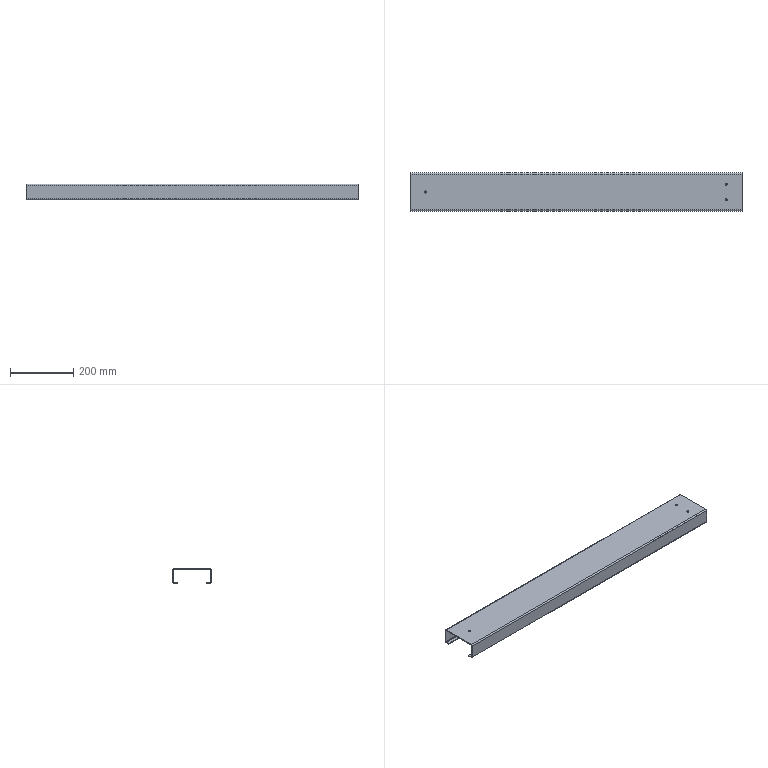Part | SolidWorks | features BaseBody 1 | 1 solid | 44 faces | box 1046 x 120 x 50 mm | volume 733077 mm3 | plane 30 | cylinder 14 | commonest cylinder face diameters 6.5 x6 2 x4 8 x4
STEP:
#1=CARTESIAN_POINT('',(469.75,25.,-3.));
#2=VERTEX_POINT('',#1);
#3=CARTESIAN_POINT('',(469.75,25.,0.));
#4=VERTEX_POINT('',#3);
#5=CARTESIAN_POINT('',(469.75,25.,-3.));
#6=DIRECTION('',(0.,0.,1.));
#7=VECTOR('',#6,1000.);
#8=LINE('',#5,#7);
#9=EDGE_CURVE('',#2,#4,#8,.T.);
#10=ORIENTED_EDGE('',*,*,#9,.F.);
#11=CARTESIAN_POINT('',(476.25,25.,-3.));
#12=VERTEX_POINT('',#11);
#13=CARTESIAN_POINT('',(473.,25.,-3.));
#14=DIRECTION('',(0.,0.,1.));
#15=DIRECTION('',(1.,0.,0.));
#16=AXIS2_PLACEMENT_3D('',#13,#14,#15);
#17=CIRCLE('',#16,3.25);
#18=EDGE_CURVE('',#12,#2,#17,.T.);
#19=ORIENTED_EDGE('',*,*,#18,.F.);
#20=CARTESIAN_POINT('',(476.25,25.,0.));
#21=VERTEX_POINT('',#20);
#22=CARTESIAN_POINT('',(476.25,25.,-3.));
#23=DIRECTION('',(0.,0.,1.));
#24=VECTOR('',#23,1000.);
#25=LINE('',#22,#24);
#26=EDGE_CURVE('',#12,#21,#25,.T.);
#27=ORIENTED_EDGE('',*,*,#26,.T.);
#28=CARTESIAN_POINT('',(473.,25.,0.));
#29=DIRECTION('',(0.,0.,1.));
#30=DIRECTION('',(1.,0.,0.));
#31=AXIS2_PLACEMENT_3D('',#28,#29,#30);
#32=CIRCLE('',#31,3.25);
#33=EDGE_CURVE('',#21,#4,#32,.T.);
#34=ORIENTED_EDGE('',*,*,#33,.T.);
#35=EDGE_LOOP('',(#10,#19,#27,#34));
#36=FACE_OUTER_BOUND('',#35,.T.);
#37=CARTESIAN_POINT('',(473.,25.,-3.));
#38=DIRECTION('',(0.,0.,1.));
#39=DIRECTION('',(1.,0.,0.));
#40=AXIS2_PLACEMENT_3D('',#37,#38,#39);
#41=CYLINDRICAL_SURFACE('',#40,3.25);
#42=ADVANCED_FACE('',(#36),#41,.F.);
#43=CARTESIAN_POINT('',(469.75,-25.,-3.));
#44=VERTEX_POINT('',#43);
#45=CARTESIAN_POINT('',(469.75,-25.,0.));
#46=VERTEX_POINT('',#45);
#47=CARTESIAN_POINT('',(469.75,-25.,-3.));
#48=DIRECTION('',(0.,0.,1.));
#49=VECTOR('',#48,1000.);
#50=LINE('',#47,#49);
#51=EDGE_CURVE('',#44,#46,#50,.T.);
#52=ORIENTED_EDGE('',*,*,#51,.F.);
#53=CARTESIAN_POINT('',(476.25,-25.,-3.));
#54=VERTEX_POINT('',#53);
#55=CARTESIAN_POINT('',(473.,-25.,-3.));
#56=DIRECTION('',(0.,0.,1.));
#57=DIRECTION('',(1.,0.,0.));
#58=AXIS2_PLACEMENT_3D('',#55,#56,#57);
#59=CIRCLE('',#58,3.25);
#60=EDGE_CURVE('',#54,#44,#59,.T.);
#61=ORIENTED_EDGE('',*,*,#60,.F.);
#62=CARTESIAN_POINT('',(476.25,-25.,0.));
#63=VERTEX_POINT('',#62);
#64=CARTESIAN_POINT('',(476.25,-25.,-3.));
#65=DIRECTION('',(0.,0.,1.));
#66=VECTOR('',#65,1000.);
#67=LINE('',#64,#66);
#68=EDGE_CURVE('',#54,#63,#67,.T.);
#69=ORIENTED_EDGE('',*,*,#68,.T.);
#70=CARTESIAN_POINT('',(473.,-25.,0.));
#71=DIRECTION('',(0.,0.,1.));
#72=DIRECTION('',(1.,0.,0.));
#73=AXIS2_PLACEMENT_3D('',#70,#71,#72);
#74=CIRCLE('',#73,3.25);
#75=EDGE_CURVE('',#63,#46,#74,.T.);
#76=ORIENTED_EDGE('',*,*,#75,.T.);
#77=EDGE_LOOP('',(#52,#61,#69,#76));
#78=FACE_OUTER_BOUND('',#77,.T.);
#79=CARTESIAN_POINT('',(473.,-25.,-3.));
#80=DIRECTION('',(0.,0.,1.));
#81=DIRECTION('',(1.,0.,0.));
#82=AXIS2_PLACEMENT_3D('',#79,#80,#81);
#83=CYLINDRICAL_SURFACE('',#82,3.25);
#84=ADVANCED_FACE('',(#78),#83,.F.);
#85=CARTESIAN_POINT('',(-476.25,0.,-3.));
#86=VERTEX_POINT('',#85);
#87=CARTESIAN_POINT('',(-476.25,0.,0.));
#88=VERTEX_POINT('',#87);
#89=CARTESIAN_POINT('',(-476.25,0.,-3.));
#90=DIRECTION('',(0.,0.,1.));
#91=VECTOR('',#90,1000.);
#92=LINE('',#89,#91);
#93=EDGE_CURVE('',#86,#88,#92,.T.);
#94=ORIENTED_EDGE('',*,*,#93,.F.);
#95=CARTESIAN_POINT('',(-469.75,0.,-3.));
#96=VERTEX_POINT('',#95);
#97=CARTESIAN_POINT('',(-473.,0.,-3.));
#98=DIRECTION('',(0.,0.,1.));
#99=DIRECTION('',(1.,0.,0.));
#100=AXIS2_PLACEMENT_3D('',#97,#98,#99);
#101=CIRCLE('',#100,3.25);
#102=EDGE_CURVE('',#96,#86,#101,.T.);
#103=ORIENTED_EDGE('',*,*,#102,.F.);
#104=CARTESIAN_POINT('',(-469.75,0.,0.));
#105=VERTEX_POINT('',#104);
#106=CARTESIAN_POINT('',(-469.75,0.,-3.));
#107=DIRECTION('',(0.,0.,1.));
#108=VECTOR('',#107,1000.);
#109=LINE('',#106,#108);
#110=EDGE_CURVE('',#96,#105,#109,.T.);
#111=ORIENTED_EDGE('',*,*,#110,.T.);
#112=CARTESIAN_POINT('',(-473.,0.,0.));
#113=DIRECTION('',(0.,0.,1.));
#114=DIRECTION('',(1.,0.,0.));
#115=AXIS2_PLACEMENT_3D('',#112,#113,#114);
#116=CIRCLE('',#115,3.25);
#117=EDGE_CURVE('',#105,#88,#116,.T.);
#118=ORIENTED_EDGE('',*,*,#117,.T.);
#119=EDGE_LOOP('',(#94,#103,#111,#118));
#120=FACE_OUTER_BOUND('',#119,.T.);
#121=CARTESIAN_POINT('',(-473.,0.,-3.));
#122=DIRECTION('',(0.,0.,1.));
#123=DIRECTION('',(1.,0.,0.));
#124=AXIS2_PLACEMENT_3D('',#121,#122,#123);
#125=CYLINDRICAL_SURFACE('',#124,3.25);
#126=ADVANCED_FACE('',(#120),#125,.F.);
#127=CARTESIAN_POINT('',(523.,45.,-47.));
#128=VERTEX_POINT('',#127);
#129=CARTESIAN_POINT('',(-523.,45.,-47.));
#130=VERTEX_POINT('',#129);
#131=CARTESIAN_POINT('',(-523.,45.,-47.));
#132=DIRECTION('',(-1.,0.,0.));
#133=VECTOR('',#132,1000.);
#134=LINE('',#131,#133);
#135=EDGE_CURVE('',#128,#130,#134,.T.);
#136=ORIENTED_EDGE('',*,*,#135,.T.);
#137=CARTESIAN_POINT('',(-523.,45.,-50.));
#138=VERTEX_POINT('',#137);
#139=CARTESIAN_POINT('',(-523.,45.,-50.));
#140=DIRECTION('',(0.,0.,1.));
#141=VECTOR('',#140,1000.);
#142=LINE('',#139,#141);
#143=EDGE_CURVE('',#138,#130,#142,.T.);
#144=ORIENTED_EDGE('',*,*,#143,.F.);
#145=CARTESIAN_POINT('',(523.,45.,-50.));
#146=VERTEX_POINT('',#145);
#147=CARTESIAN_POINT('',(0.,45.,-50.));
#148=DIRECTION('',(-1.,0.,0.));
#149=VECTOR('',#148,1000.);
#150=LINE('',#147,#149);
#151=EDGE_CURVE('',#146,#138,#150,.T.);
#152=ORIENTED_EDGE('',*,*,#151,.F.);
#153=CARTESIAN_POINT('',(523.,45.,-50.));
#154=DIRECTION('',(0.,0.,1.));
#155=VECTOR('',#154,1000.);
#156=LINE('',#153,#155);
#157=EDGE_CURVE('',#146,#128,#156,.T.);
#158=ORIENTED_EDGE('',*,*,#157,.T.);
#159=EDGE_LOOP('',(#136,#144,#152,#158));
#160=FACE_OUTER_BOUND('',#159,.T.);
#161=CARTESIAN_POINT('',(-523.,45.,-50.));
#162=DIRECTION('',(0.,1.,0.));
#163=DIRECTION('',(0.,0.,-1.));
#164=AXIS2_PLACEMENT_3D('',#161,#162,#163);
#165=PLANE('',#164);
#166=ADVANCED_FACE('',(#160),#165,.F.);
#167=CARTESIAN_POINT('',(523.,56.,-47.));
#168=VERTEX_POINT('',#167);
#169=CARTESIAN_POINT('',(523.,45.,-47.));
#170=DIRECTION('',(0.,-1.,0.));
#171=VECTOR('',#170,1000.);
#172=LINE('',#169,#171);
#173=EDGE_CURVE('',#168,#128,#172,.T.);
#174=ORIENTED_EDGE('',*,*,#173,.F.);
#175=CARTESIAN_POINT('',(-523.,56.,-47.));
#176=VERTEX_POINT('',#175);
#177=CARTESIAN_POINT('',(-523.,56.,-47.));
#178=DIRECTION('',(1.,0.,0.));
#179=VECTOR('',#178,1000.);
#180=LINE('',#177,#179);
#181=EDGE_CURVE('',#176,#168,#180,.T.);
#182=ORIENTED_EDGE('',*,*,#181,.F.);
#183=CARTESIAN_POINT('',(-523.,57.,-47.));
#184=DIRECTION('',(0.,1.,0.));
#185=VECTOR('',#184,1000.);
#186=LINE('',#183,#185);
#187=EDGE_CURVE('',#130,#176,#186,.T.);
#188=ORIENTED_EDGE('',*,*,#187,.F.);
#189=ORIENTED_EDGE('',*,*,#135,.F.);
#190=EDGE_LOOP('',(#174,#182,#188,#189));
#191=FACE_OUTER_BOUND('',#190,.T.);
#192=CARTESIAN_POINT('',(0.,0.,-47.));
#193=DIRECTION('',(0.,0.,1.));
#194=DIRECTION('',(0.,-1.,0.));
#195=AXIS2_PLACEMENT_3D('',#192,#193,#194);
#196=PLANE('',#195);
#197=ADVANCED_FACE('',(#191),#196,.T.);
#198=CARTESIAN_POINT('',(523.,56.,-50.));
#199=VERTEX_POINT('',#198);
#200=CARTESIAN_POINT('',(-523.,56.,-50.));
#201=VERTEX_POINT('',#200);
#202=CARTESIAN_POINT('',(-523.,56.,-50.));
#203=DIRECTION('',(-1.,0.,0.));
#204=VECTOR('',#203,1000.);
#205=LINE('',#202,#204);
#206=EDGE_CURVE('',#199,#201,#205,.T.);
#207=ORIENTED_EDGE('',*,*,#206,.F.);
#208=CARTESIAN_POINT('',(523.,0.,-50.));
#209=DIRECTION('',(0.,-1.,0.));
#210=VECTOR('',#209,1000.);
#211=LINE('',#208,#210);
#212=EDGE_CURVE('',#199,#146,#211,.T.);
#213=ORIENTED_EDGE('',*,*,#212,.T.);
#214=ORIENTED_EDGE('',*,*,#151,.T.);
#215=CARTESIAN_POINT('',(-523.,0.,-50.));
#216=DIRECTION('',(0.,1.,0.));
#217=VECTOR('',#216,1000.);
#218=LINE('',#215,#217);
#219=EDGE_CURVE('',#138,#201,#218,.T.);
#220=ORIENTED_EDGE('',*,*,#219,.T.);
#221=EDGE_LOOP('',(#207,#213,#214,#220));
#222=FACE_OUTER_BOUND('',#221,.T.);
#223=CARTESIAN_POINT('',(0.,0.,-50.));
#224=DIRECTION('',(0.,0.,1.));
#225=DIRECTION('',(0.,-1.,0.));
#226=AXIS2_PLACEMENT_3D('',#223,#224,#225);
#227=PLANE('',#226);
#228=ADVANCED_FACE('',(#222),#227,.F.);
#229=CARTESIAN_POINT('',(-523.,56.,-50.));
#230=DIRECTION('',(0.,0.,-1.));
#231=VECTOR('',#230,1000.);
#232=LINE('',#229,#231);
#233=EDGE_CURVE('',#176,#201,#232,.T.);
#234=ORIENTED_EDGE('',*,*,#233,.T.);
#235=ORIENTED_EDGE('',*,*,#219,.F.);
#236=ORIENTED_EDGE('',*,*,#143,.T.);
#237=ORIENTED_EDGE('',*,*,#187,.T.);
#238=EDGE_LOOP('',(#234,#235,#236,#237));
#239=FACE_OUTER_BOUND('',#238,.T.);
#240=CARTESIAN_POINT('',(-523.,57.,-50.));
#241=DIRECTION('',(1.,0.,0.));
#242=DIRECTION('',(0.,1.,0.));
#243=AXIS2_PLACEMENT_3D('',#240,#241,#242);
#244=PLANE('',#243);
#245=ADVANCED_FACE('',(#239),#244,.F.);
#246=CARTESIAN_POINT('',(523.,56.,-47.));
#247=DIRECTION('',(0.,0.,-1.));
#248=VECTOR('',#247,1000.);
#249=LINE('',#246,#248);
#250=EDGE_CURVE('',#168,#199,#249,.T.);
#251=ORIENTED_EDGE('',*,*,#250,.F.);
#252=ORIENTED_EDGE('',*,*,#173,.T.);
#253=ORIENTED_EDGE('',*,*,#157,.F.);
#254=ORIENTED_EDGE('',*,*,#212,.F.);
#255=EDGE_LOOP('',(#251,#252,#253,#254));
#256=FACE_OUTER_BOUND('',#255,.T.);
#257=CARTESIAN_POINT('',(523.,45.,-50.));
#258=DIRECTION('',(-1.,0.,0.));
#259=DIRECTION('',(0.,0.,1.));
#260=AXIS2_PLACEMENT_3D('',#257,#258,#259);
#261=PLANE('',#260);
#262=ADVANCED_FACE('',(#256),#261,.F.);
#263=CARTESIAN_POINT('',(523.,57.,-46.));
#264=VERTEX_POINT('',#263);
#265=CARTESIAN_POINT('',(-523.,57.,-46.));
#266=VERTEX_POINT('',#265);
#267=CARTESIAN_POINT('',(523.,57.,-46.));
#268=DIRECTION('',(-1.,0.,0.));
#269=VECTOR('',#268,1000.);
#270=LINE('',#267,#269);
#271=EDGE_CURVE('',#264,#266,#270,.T.);
#272=ORIENTED_EDGE('',*,*,#271,.T.);
#273=CARTESIAN_POINT('',(-523.,56.,-46.));
#274=DIRECTION('',(-1.,0.,0.));
#275=DIRECTION('',(0.,0.,-1.));
#276=AXIS2_PLACEMENT_3D('',#273,#274,#275);
#277=CIRCLE('',#276,1.);
#278=EDGE_CURVE('',#266,#176,#277,.T.);
#279=ORIENTED_EDGE('',*,*,#278,.T.);
#280=ORIENTED_EDGE('',*,*,#181,.T.);
#281=CARTESIAN_POINT('',(523.,56.,-46.));
#282=DIRECTION('',(1.,0.,0.));
#283=DIRECTION('',(0.,0.,-1.));
#284=AXIS2_PLACEMENT_3D('',#281,#282,#283);
#285=CIRCLE('',#284,1.);
#286=EDGE_CURVE('',#168,#264,#285,.T.);
#287=ORIENTED_EDGE('',*,*,#286,.T.);
#288=EDGE_LOOP('',(#272,#279,#280,#287));
#289=FACE_OUTER_BOUND('',#288,.T.);
#290=CARTESIAN_POINT('',(523.,56.,-46.));
#291=DIRECTION('',(1.,0.,0.));
#292=DIRECTION('',(0.,0.,-1.));
#293=AXIS2_PLACEMENT_3D('',#290,#291,#292);
#294=CYLINDRICAL_SURFACE('',#293,1.);
#295=ADVANCED_FACE('',(#289),#294,.F.);
#296=CARTESIAN_POINT('',(523.,60.,-46.));
#297=VERTEX_POINT('',#296);
#298=CARTESIAN_POINT('',(-523.,60.,-46.));
#299=VERTEX_POINT('',#298);
#300=CARTESIAN_POINT('',(523.,60.,-46.));
#301=DIRECTION('',(-1.,0.,0.));
#302=VECTOR('',#301,1000.);
#303=LINE('',#300,#302);
#304=EDGE_CURVE('',#297,#299,#303,.T.);
#305=ORIENTED_EDGE('',*,*,#304,.F.);
#306=CARTESIAN_POINT('',(523.,56.,-46.));
#307=DIRECTION('',(1.,0.,0.));
#308=DIRECTION('',(0.,0.,-1.));
#309=AXIS2_PLACEMENT_3D('',#306,#307,#308);
#310=CIRCLE('',#309,4.);
#311=EDGE_CURVE('',#199,#297,#310,.T.);
#312=ORIENTED_EDGE('',*,*,#311,.F.);
#313=ORIENTED_EDGE('',*,*,#206,.T.);
#314=CARTESIAN_POINT('',(-523.,56.,-46.));
#315=DIRECTION('',(-1.,0.,0.));
#316=DIRECTION('',(0.,0.,-1.));
#317=AXIS2_PLACEMENT_3D('',#314,#315,#316);
#318=CIRCLE('',#317,4.);
#319=EDGE_CURVE('',#299,#201,#318,.T.);
#320=ORIENTED_EDGE('',*,*,#319,.F.);
#321=EDGE_LOOP('',(#305,#312,#313,#320));
#322=FACE_OUTER_BOUND('',#321,.T.);
#323=CARTESIAN_POINT('',(523.,56.,-46.));
#324=DIRECTION('',(1.,0.,0.));
#325=DIRECTION('',(0.,0.,-1.));
#326=AXIS2_PLACEMENT_3D('',#323,#324,#325);
#327=CYLINDRICAL_SURFACE('',#326,4.);
#328=ADVANCED_FACE('',(#322),#327,.T.);
#329=ORIENTED_EDGE('',*,*,#286,.F.);
#330=ORIENTED_EDGE('',*,*,#250,.T.);
#331=ORIENTED_EDGE('',*,*,#311,.T.);
#332=CARTESIAN_POINT('',(523.,57.,-46.));
#333=DIRECTION('',(0.,1.,0.));
#334=VECTOR('',#333,1000.);
#335=LINE('',#332,#334);
#336=EDGE_CURVE('',#264,#297,#335,.T.);
#337=ORIENTED_EDGE('',*,*,#336,.F.);
#338=EDGE_LOOP('',(#329,#330,#331,#337));
#339=FACE_OUTER_BOUND('',#338,.T.);
#340=CARTESIAN_POINT('',(523.,56.,-46.));
#341=DIRECTION('',(-1.,0.,0.));
#342=DIRECTION('',(0.,0.,1.));
#343=AXIS2_PLACEMENT_3D('',#340,#341,#342);
#344=PLANE('',#343);
#345=ADVANCED_FACE('',(#339),#344,.F.);
#346=ORIENTED_EDGE('',*,*,#233,.F.);
#347=ORIENTED_EDGE('',*,*,#278,.F.);
#348=CARTESIAN_POINT('',(-523.,57.,-46.));
#349=DIRECTION('',(0.,1.,0.));
#350=VECTOR('',#349,1000.);
#351=LINE('',#348,#350);
#352=EDGE_CURVE('',#266,#299,#351,.T.);
#353=ORIENTED_EDGE('',*,*,#352,.T.);
#354=ORIENTED_EDGE('',*,*,#319,.T.);
#355=EDGE_LOOP('',(#346,#347,#353,#354));
#356=FACE_OUTER_BOUND('',#355,.T.);
#357=CARTESIAN_POINT('',(-523.,56.,-46.));
#358=DIRECTION('',(-1.,0.,0.));
#359=DIRECTION('',(0.,0.,1.));
#360=AXIS2_PLACEMENT_3D('',#357,#358,#359);
#361=PLANE('',#360);
#362=ADVANCED_FACE('',(#356),#361,.T.);
#363=CARTESIAN_POINT('',(-523.,-45.,-47.));
#364=VERTEX_POINT('',#363);
#365=CARTESIAN_POINT('',(523.,-45.,-47.));
#366=VERTEX_POINT('',#365);
#367=CARTESIAN_POINT('',(523.,-45.,-47.));
#368=DIRECTION('',(1.,0.,0.));
#369=VECTOR('',#368,1000.);
#370=LINE('',#367,#369);
#371=EDGE_CURVE('',#364,#366,#370,.T.);
#372=ORIENTED_EDGE('',*,*,#371,.T.);
#373=CARTESIAN_POINT('',(523.,-45.,-50.));
#374=VERTEX_POINT('',#373);
#375=CARTESIAN_POINT('',(523.,-45.,-50.));
#376=DIRECTION('',(0.,0.,1.));
#377=VECTOR('',#376,1000.);
#378=LINE('',#375,#377);
#379=EDGE_CURVE('',#374,#366,#378,.T.);
#380=ORIENTED_EDGE('',*,*,#379,.F.);
#381=CARTESIAN_POINT('',(-523.,-45.,-50.));
#382=VERTEX_POINT('',#381);
#383=CARTESIAN_POINT('',(0.,-45.,-50.));
#384=DIRECTION('',(1.,0.,0.));
#385=VECTOR('',#384,1000.);
#386=LINE('',#383,#385);
#387=EDGE_CURVE('',#382,#374,#386,.T.);
#388=ORIENTED_EDGE('',*,*,#387,.F.);
#389=CARTESIAN_POINT('',(-523.,-45.,-50.));
#390=DIRECTION('',(0.,0.,1.));
#391=VECTOR('',#390,1000.);
#392=LINE('',#389,#391);
#393=EDGE_CURVE('',#382,#364,#392,.T.);
#394=ORIENTED_EDGE('',*,*,#393,.T.);
#395=EDGE_LOOP('',(#372,#380,#388,#394));
#396=FACE_OUTER_BOUND('',#395,.T.);
#397=CARTESIAN_POINT('',(523.,-45.,-50.));
#398=DIRECTION('',(0.,-1.,0.));
#399=DIRECTION('',(-1.,0.,0.));
#400=AXIS2_PLACEMENT_3D('',#397,#398,#399);
#401=PLANE('',#400);
#402=ADVANCED_FACE('',(#396),#401,.F.);
#403=CARTESIAN_POINT('',(-523.,-56.,-47.));
#404=VERTEX_POINT('',#403);
#405=CARTESIAN_POINT('',(-523.,-45.,-47.));
#406=DIRECTION('',(0.,1.,0.));
#407=VECTOR('',#406,1000.);
#408=LINE('',#405,#407);
#409=EDGE_CURVE('',#404,#364,#408,.T.);
#410=ORIENTED_EDGE('',*,*,#409,.F.);
#411=CARTESIAN_POINT('',(523.,-56.,-47.));
#412=VERTEX_POINT('',#411);
#413=CARTESIAN_POINT('',(523.,-56.,-47.));
#414=DIRECTION('',(-1.,0.,0.));
#415=VECTOR('',#414,1000.);
#416=LINE('',#413,#415);
#417=EDGE_CURVE('',#412,#404,#416,.T.);
#418=ORIENTED_EDGE('',*,*,#417,.F.);
#419=CARTESIAN_POINT('',(523.,-57.,-47.));
#420=DIRECTION('',(0.,-1.,0.));
#421=VECTOR('',#420,1000.);
#422=LINE('',#419,#421);
#423=EDGE_CURVE('',#366,#412,#422,.T.);
#424=ORIENTED_EDGE('',*,*,#423,.F.);
#425=ORIENTED_EDGE('',*,*,#371,.F.);
#426=EDGE_LOOP('',(#410,#418,#424,#425));
#427=FACE_OUTER_BOUND('',#426,.T.);
#428=CARTESIAN_POINT('',(0.,0.,-47.));
#429=DIRECTION('',(0.,0.,1.));
#430=DIRECTION('',(0.,-1.,0.));
#431=AXIS2_PLACEMENT_3D('',#428,#429,#430);
#432=PLANE('',#431);
#433=ADVANCED_FACE('',(#427),#432,.T.);
#434=CARTESIAN_POINT('',(-523.,-56.,-50.));
#435=VERTEX_POINT('',#434);
#436=CARTESIAN_POINT('',(523.,-56.,-50.));
#437=VERTEX_POINT('',#436);
#438=CARTESIAN_POINT('',(523.,-56.,-50.));
#439=DIRECTION('',(1.,0.,0.));
#440=VECTOR('',#439,1000.);
#441=LINE('',#438,#440);
#442=EDGE_CURVE('',#435,#437,#441,.T.);
#443=ORIENTED_EDGE('',*,*,#442,.F.);
#444=CARTESIAN_POINT('',(-523.,0.,-50.));
#445=DIRECTION('',(0.,1.,0.));
#446=VECTOR('',#445,1000.);
#447=LINE('',#444,#446);
#448=EDGE_CURVE('',#435,#382,#447,.T.);
#449=ORIENTED_EDGE('',*,*,#448,.T.);
#450=ORIENTED_EDGE('',*,*,#387,.T.);
#451=CARTESIAN_POINT('',(523.,0.,-50.));
#452=DIRECTION('',(0.,-1.,0.));
#453=VECTOR('',#452,1000.);
#454=LINE('',#451,#453);
#455=EDGE_CURVE('',#374,#437,#454,.T.);
#456=ORIENTED_EDGE('',*,*,#455,.T.);
#457=EDGE_LOOP('',(#443,#449,#450,#456));
#458=FACE_OUTER_BOUND('',#457,.T.);
#459=CARTESIAN_POINT('',(0.,0.,-50.));
#460=DIRECTION('',(0.,0.,1.));
#461=DIRECTION('',(0.,-1.,0.));
#462=AXIS2_PLACEMENT_3D('',#459,#460,#461);
#463=PLANE('',#462);
#464=ADVANCED_FACE('',(#458),#463,.F.);
#465=CARTESIAN_POINT('',(523.,-56.,-50.));
#466=DIRECTION('',(0.,0.,-1.));
#467=VECTOR('',#466,1000.);
#468=LINE('',#465,#467);
#469=EDGE_CURVE('',#412,#437,#468,.T.);
#470=ORIENTED_EDGE('',*,*,#469,.T.);
#471=ORIENTED_EDGE('',*,*,#455,.F.);
#472=ORIENTED_EDGE('',*,*,#379,.T.);
#473=ORIENTED_EDGE('',*,*,#423,.T.);
#474=EDGE_LOOP('',(#470,#471,#472,#473));
#475=FACE_OUTER_BOUND('',#474,.T.);
#476=CARTESIAN_POINT('',(523.,-57.,-50.));
#477=DIRECTION('',(-1.,0.,0.));
#478=DIRECTION('',(0.,0.,1.));
#479=AXIS2_PLACEMENT_3D('',#476,#477,#478);
#480=PLANE('',#479);
#481=ADVANCED_FACE('',(#475),#480,.F.);
#482=CARTESIAN_POINT('',(-523.,-56.,-47.));
#483=DIRECTION('',(0.,0.,-1.));
#484=VECTOR('',#483,1000.);
#485=LINE('',#482,#484);
#486=EDGE_CURVE('',#404,#435,#485,.T.);
#487=ORIENTED_EDGE('',*,*,#486,.F.);
#488=ORIENTED_EDGE('',*,*,#409,.T.);
#489=ORIENTED_EDGE('',*,*,#393,.F.);
#490=ORIENTED_EDGE('',*,*,#448,.F.);
#491=EDGE_LOOP('',(#487,#488,#489,#490));
#492=FACE_OUTER_BOUND('',#491,.T.);
#493=CARTESIAN_POINT('',(-523.,-45.,-50.));
#494=DIRECTION('',(1.,0.,0.));
#495=DIRECTION('',(0.,1.,0.));
#496=AXIS2_PLACEMENT_3D('',#493,#494,#495);
#497=PLANE('',#496);
#498=ADVANCED_FACE('',(#492),#497,.F.);
#499=CARTESIAN_POINT('',(-523.,-57.,-46.));
#500=VERTEX_POINT('',#499);
#501=CARTESIAN_POINT('',(523.,-57.,-46.));
#502=VERTEX_POINT('',#501);
#503=CARTESIAN_POINT('',(-523.,-57.,-46.));
#504=DIRECTION('',(1.,0.,0.));
#505=VECTOR('',#504,1000.);
#506=LINE('',#503,#505);
#507=EDGE_CURVE('',#500,#502,#506,.T.);
#508=ORIENTED_EDGE('',*,*,#507,.T.);
#509=CARTESIAN_POINT('',(523.,-56.,-46.));
#510=DIRECTION('',(1.,0.,0.));
#511=DIRECTION('',(0.,0.,1.));
#512=AXIS2_PLACEMENT_3D('',#509,#510,#511);
#513=CIRCLE('',#512,1.);
#514=EDGE_CURVE('',#502,#412,#513,.T.);
#515=ORIENTED_EDGE('',*,*,#514,.T.);
#516=ORIENTED_EDGE('',*,*,#417,.T.);
#517=CARTESIAN_POINT('',(-523.,-56.,-46.));
#518=DIRECTION('',(-1.,0.,0.));
#519=DIRECTION('',(0.,0.,1.));
#520=AXIS2_PLACEMENT_3D('',#517,#518,#519);
#521=CIRCLE('',#520,1.);
#522=EDGE_CURVE('',#404,#500,#521,.T.);
#523=ORIENTED_EDGE('',*,*,#522,.T.);
#524=EDGE_LOOP('',(#508,#515,#516,#523));
#525=FACE_OUTER_BOUND('',#524,.T.);
#526=CARTESIAN_POINT('',(-523.,-56.,-46.));
#527=DIRECTION('',(-1.,0.,0.));
#528=DIRECTION('',(0.,0.,-1.));
#529=AXIS2_PLACEMENT_3D('',#526,#527,#528);
#530=CYLINDRICAL_SURFACE('',#529,1.);
#531=ADVANCED_FACE('',(#525),#530,.F.);
#532=CARTESIAN_POINT('',(-523.,-60.,-46.));
#533=VERTEX_POINT('',#532);
#534=CARTESIAN_POINT('',(523.,-60.,-46.));
#535=VERTEX_POINT('',#534);
#536=CARTESIAN_POINT('',(-523.,-60.,-46.));
#537=DIRECTION('',(1.,0.,0.));
#538=VECTOR('',#537,1000.);
#539=LINE('',#536,#538);
#540=EDGE_CURVE('',#533,#535,#539,.T.);
#541=ORIENTED_EDGE('',*,*,#540,.F.);
#542=CARTESIAN_POINT('',(-523.,-56.,-46.));
#543=DIRECTION('',(-1.,0.,0.));
#544=DIRECTION('',(0.,0.,1.));
#545=AXIS2_PLACEMENT_3D('',#542,#543,#544);
#546=CIRCLE('',#545,4.);
#547=EDGE_CURVE('',#435,#533,#546,.T.);
#548=ORIENTED_EDGE('',*,*,#547,.F.);
#549=ORIENTED_EDGE('',*,*,#442,.T.);
#550=CARTESIAN_POINT('',(523.,-56.,-46.));
#551=DIRECTION('',(1.,0.,0.));
#552=DIRECTION('',(0.,0.,1.));
#553=AXIS2_PLACEMENT_3D('',#550,#551,#552);
#554=CIRCLE('',#553,4.);
#555=EDGE_CURVE('',#535,#437,#554,.T.);
#556=ORIENTED_EDGE('',*,*,#555,.F.);
#557=EDGE_LOOP('',(#541,#548,#549,#556));
#558=FACE_OUTER_BOUND('',#557,.T.);
#559=CARTESIAN_POINT('',(-523.,-56.,-46.));
#560=DIRECTION('',(-1.,0.,0.));
#561=DIRECTION('',(0.,0.,-1.));
#562=AXIS2_PLACEMENT_3D('',#559,#560,#561);
#563=CYLINDRICAL_SURFACE('',#562,4.);
#564=ADVANCED_FACE('',(#558),#563,.T.);
#565=ORIENTED_EDGE('',*,*,#522,.F.);
#566=ORIENTED_EDGE('',*,*,#486,.T.);
#567=ORIENTED_EDGE('',*,*,#547,.T.);
#568=CARTESIAN_POINT('',(-523.,-57.,-46.));
#569=DIRECTION('',(0.,-1.,0.));
#570=VECTOR('',#569,1000.);
#571=LINE('',#568,#570);
#572=EDGE_CURVE('',#500,#533,#571,.T.);
#573=ORIENTED_EDGE('',*,*,#572,.F.);
#574=EDGE_LOOP('',(#565,#566,#567,#573));
#575=FACE_OUTER_BOUND('',#574,.T.);
#576=CARTESIAN_POINT('',(-523.,-56.,-46.));
#577=DIRECTION('',(1.,0.,0.));
#578=DIRECTION('',(0.,1.,0.));
#579=AXIS2_PLACEMENT_3D('',#576,#577,#578);
#580=PLANE('',#579);
#581=ADVANCED_FACE('',(#575),#580,.F.);
#582=ORIENTED_EDGE('',*,*,#469,.F.);
#583=ORIENTED_EDGE('',*,*,#514,.F.);
#584=CARTESIAN_POINT('',(523.,-57.,-46.));
#585=DIRECTION('',(0.,-1.,0.));
#586=VECTOR('',#585,1000.);
#587=LINE('',#584,#586);
#588=EDGE_CURVE('',#502,#535,#587,.T.);
#589=ORIENTED_EDGE('',*,*,#588,.T.);
#590=ORIENTED_EDGE('',*,*,#555,.T.);
#591=EDGE_LOOP('',(#582,#583,#589,#590));
#592=FACE_OUTER_BOUND('',#591,.T.);
#593=CARTESIAN_POINT('',(523.,-56.,-46.));
#594=DIRECTION('',(1.,0.,0.));
#595=DIRECTION('',(0.,1.,0.));
#596=AXIS2_PLACEMENT_3D('',#593,#594,#595);
#597=PLANE('',#596);
#598=ADVANCED_FACE('',(#592),#597,.T.);
#599=CARTESIAN_POINT('',(523.,56.,-3.));
#600=VERTEX_POINT('',#599);
#601=CARTESIAN_POINT('',(-523.,56.,-3.));
#602=VERTEX_POINT('',#601);
#603=CARTESIAN_POINT('',(523.,56.,-3.));
#604=DIRECTION('',(-1.,0.,0.));
#605=VECTOR('',#604,1000.);
#606=LINE('',#603,#605);
#607=EDGE_CURVE('',#600,#602,#606,.T.);
#608=ORIENTED_EDGE('',*,*,#607,.T.);
#609=CARTESIAN_POINT('',(-523.,57.,-4.));
#610=VERTEX_POINT('',#609);
#611=CARTESIAN_POINT('',(-523.,56.,-4.));
#612=DIRECTION('',(-1.,0.,0.));
#613=DIRECTION('',(0.,0.,-1.));
#614=AXIS2_PLACEMENT_3D('',#611,#612,#613);
#615=CIRCLE('',#614,1.);
#616=EDGE_CURVE('',#602,#610,#615,.T.);
#617=ORIENTED_EDGE('',*,*,#616,.T.);
#618=CARTESIAN_POINT('',(523.,57.,-4.));
#619=VERTEX_POINT('',#618);
#620=CARTESIAN_POINT('',(-523.,57.,-4.));
#621=DIRECTION('',(1.,0.,0.));
#622=VECTOR('',#621,1000.);
#623=LINE('',#620,#622);
#624=EDGE_CURVE('',#610,#619,#623,.T.);
#625=ORIENTED_EDGE('',*,*,#624,.T.);
#626=CARTESIAN_POINT('',(523.,56.,-4.));
#627=DIRECTION('',(1.,0.,0.));
#628=DIRECTION('',(0.,0.,-1.));
#629=AXIS2_PLACEMENT_3D('',#626,#627,#628);
#630=CIRCLE('',#629,1.);
#631=EDGE_CURVE('',#619,#600,#630,.T.);
#632=ORIENTED_EDGE('',*,*,#631,.T.);
#633=EDGE_LOOP('',(#608,#617,#625,#632));
#634=FACE_OUTER_BOUND('',#633,.T.);
#635=CARTESIAN_POINT('',(523.,56.,-4.));
#636=DIRECTION('',(1.,0.,0.));
#637=DIRECTION('',(0.,1.,0.));
#638=AXIS2_PLACEMENT_3D('',#635,#636,#637);
#639=CYLINDRICAL_SURFACE('',#638,1.);
#640=ADVANCED_FACE('',(#634),#639,.F.);
#641=CARTESIAN_POINT('',(523.,56.,0.));
#642=VERTEX_POINT('',#641);
#643=CARTESIAN_POINT('',(-523.,56.,0.));
#644=VERTEX_POINT('',#643);
#645=CARTESIAN_POINT('',(523.,56.,0.));
#646=DIRECTION('',(-1.,0.,0.));
#647=VECTOR('',#646,1000.);
#648=LINE('',#645,#647);
#649=EDGE_CURVE('',#642,#644,#648,.T.);
#650=ORIENTED_EDGE('',*,*,#649,.F.);
#651=CARTESIAN_POINT('',(523.,60.,-4.));
#652=VERTEX_POINT('',#651);
#653=CARTESIAN_POINT('',(523.,56.,-4.));
#654=DIRECTION('',(1.,0.,0.));
#655=DIRECTION('',(0.,0.,-1.));
#656=AXIS2_PLACEMENT_3D('',#653,#654,#655);
#657=CIRCLE('',#656,4.);
#658=EDGE_CURVE('',#652,#642,#657,.T.);
#659=ORIENTED_EDGE('',*,*,#658,.F.);
#660=CARTESIAN_POINT('',(-523.,60.,-4.));
#661=VERTEX_POINT('',#660);
#662=CARTESIAN_POINT('',(-523.,60.,-4.));
#663=DIRECTION('',(-1.,0.,0.));
#664=VECTOR('',#663,1000.);
#665=LINE('',#662,#664);
#666=EDGE_CURVE('',#652,#661,#665,.T.);
#667=ORIENTED_EDGE('',*,*,#666,.T.);
#668=CARTESIAN_POINT('',(-523.,56.,-4.));
#669=DIRECTION('',(-1.,0.,0.));
#670=DIRECTION('',(0.,0.,-1.));
#671=AXIS2_PLACEMENT_3D('',#668,#669,#670);
#672=CIRCLE('',#671,4.);
#673=EDGE_CURVE('',#644,#661,#672,.T.);
#674=ORIENTED_EDGE('',*,*,#673,.F.);
#675=EDGE_LOOP('',(#650,#659,#667,#674));
#676=FACE_OUTER_BOUND('',#675,.T.);
#677=CARTESIAN_POINT('',(523.,56.,-4.));
#678=DIRECTION('',(1.,0.,0.));
#679=DIRECTION('',(0.,1.,0.));
#680=AXIS2_PLACEMENT_3D('',#677,#678,#679);
#681=CYLINDRICAL_SURFACE('',#680,4.);
#682=ADVANCED_FACE('',(#676),#681,.T.);
#683=ORIENTED_EDGE('',*,*,#631,.F.);
#684=CARTESIAN_POINT('',(523.,57.,-4.));
#685=DIRECTION('',(0.,1.,0.));
#686=VECTOR('',#685,1000.);
#687=LINE('',#684,#686);
#688=EDGE_CURVE('',#619,#652,#687,.T.);
#689=ORIENTED_EDGE('',*,*,#688,.T.);
#690=ORIENTED_EDGE('',*,*,#658,.T.);
#691=CARTESIAN_POINT('',(523.,56.,-3.));
#692=DIRECTION('',(0.,0.,1.));
#693=VECTOR('',#692,1000.);
#694=LINE('',#691,#693);
#695=EDGE_CURVE('',#600,#642,#694,.T.);
#696=ORIENTED_EDGE('',*,*,#695,.F.);
#697=EDGE_LOOP('',(#683,#689,#690,#696));
#698=FACE_OUTER_BOUND('',#697,.T.);
#699=CARTESIAN_POINT('',(523.,56.,-4.));
#700=DIRECTION('',(-1.,0.,0.));
#701=DIRECTION('',(0.,0.,1.));
#702=AXIS2_PLACEMENT_3D('',#699,#700,#701);
#703=PLANE('',#702);
#704=ADVANCED_FACE('',(#698),#703,.F.);
#705=CARTESIAN_POINT('',(-523.,60.,-4.));
#706=DIRECTION('',(0.,1.,0.));
#707=VECTOR('',#706,1000.);
#708=LINE('',#705,#707);
#709=EDGE_CURVE('',#610,#661,#708,.T.);
#710=ORIENTED_EDGE('',*,*,#709,.F.);
#711=ORIENTED_EDGE('',*,*,#616,.F.);
#712=CARTESIAN_POINT('',(-523.,56.,-3.));
#713=DIRECTION('',(0.,0.,1.));
#714=VECTOR('',#713,1000.);
#715=LINE('',#712,#714);
#716=EDGE_CURVE('',#602,#644,#715,.T.);
#717=ORIENTED_EDGE('',*,*,#716,.T.);
#718=ORIENTED_EDGE('',*,*,#673,.T.);
#719=EDGE_LOOP('',(#710,#711,#717,#718));
#720=FACE_OUTER_BOUND('',#719,.T.);
#721=CARTESIAN_POINT('',(-523.,56.,-4.));
#722=DIRECTION('',(-1.,0.,0.));
#723=DIRECTION('',(0.,0.,1.));
#724=AXIS2_PLACEMENT_3D('',#721,#722,#723);
#725=PLANE('',#724);
#726=ADVANCED_FACE('',(#720),#725,.T.);
#727=CARTESIAN_POINT('',(-523.,-56.,-3.));
#728=VERTEX_POINT('',#727);
#729=CARTESIAN_POINT('',(523.,-56.,-3.));
#730=VERTEX_POINT('',#729);
#731=CARTESIAN_POINT('',(-523.,-56.,-3.));
#732=DIRECTION('',(1.,0.,0.));
#733=VECTOR('',#732,1000.);
#734=LINE('',#731,#733);
#735=EDGE_CURVE('',#728,#730,#734,.T.);
#736=ORIENTED_EDGE('',*,*,#735,.T.);
#737=CARTESIAN_POINT('',(523.,-57.,-4.));
#738=VERTEX_POINT('',#737);
#739=CARTESIAN_POINT('',(523.,-56.,-4.));
#740=DIRECTION('',(1.,0.,0.));
#741=DIRECTION('',(0.,0.,1.));
#742=AXIS2_PLACEMENT_3D('',#739,#740,#741);
#743=CIRCLE('',#742,1.);
#744=EDGE_CURVE('',#730,#738,#743,.T.);
#745=ORIENTED_EDGE('',*,*,#744,.T.);
#746=CARTESIAN_POINT('',(-523.,-57.,-4.));
#747=VERTEX_POINT('',#746);
#748=CARTESIAN_POINT('',(523.,-57.,-4.));
#749=DIRECTION('',(-1.,0.,0.));
#750=VECTOR('',#749,1000.);
#751=LINE('',#748,#750);
#752=EDGE_CURVE('',#738,#747,#751,.T.);
#753=ORIENTED_EDGE('',*,*,#752,.T.);
#754=CARTESIAN_POINT('',(-523.,-56.,-4.));
#755=DIRECTION('',(-1.,0.,0.));
#756=DIRECTION('',(0.,0.,1.));
#757=AXIS2_PLACEMENT_3D('',#754,#755,#756);
#758=CIRCLE('',#757,1.);
#759=EDGE_CURVE('',#747,#728,#758,.T.);
#760=ORIENTED_EDGE('',*,*,#759,.T.);
#761=EDGE_LOOP('',(#736,#745,#753,#760));
#762=FACE_OUTER_BOUND('',#761,.T.);
#763=CARTESIAN_POINT('',(-523.,-56.,-4.));
#764=DIRECTION('',(-1.,0.,0.));
#765=DIRECTION('',(0.,-1.,0.));
#766=AXIS2_PLACEMENT_3D('',#763,#764,#765);
#767=CYLINDRICAL_SURFACE('',#766,1.);
#768=ADVANCED_FACE('',(#762),#767,.F.);
#769=CARTESIAN_POINT('',(-523.,-56.,0.));
#770=VERTEX_POINT('',#769);
#771=CARTESIAN_POINT('',(523.,-56.,0.));
#772=VERTEX_POINT('',#771);
#773=CARTESIAN_POINT('',(-523.,-56.,0.));
#774=DIRECTION('',(1.,0.,0.));
#775=VECTOR('',#774,1000.);
#776=LINE('',#773,#775);
#777=EDGE_CURVE('',#770,#772,#776,.T.);
#778=ORIENTED_EDGE('',*,*,#777,.F.);
#779=CARTESIAN_POINT('',(-523.,-60.,-4.));
#780=VERTEX_POINT('',#779);
#781=CARTESIAN_POINT('',(-523.,-56.,-4.));
#782=DIRECTION('',(-1.,0.,0.));
#783=DIRECTION('',(0.,0.,1.));
#784=AXIS2_PLACEMENT_3D('',#781,#782,#783);
#785=CIRCLE('',#784,4.);
#786=EDGE_CURVE('',#780,#770,#785,.T.);
#787=ORIENTED_EDGE('',*,*,#786,.F.);
#788=CARTESIAN_POINT('',(523.,-60.,-4.));
#789=VERTEX_POINT('',#788);
#790=CARTESIAN_POINT('',(523.,-60.,-4.));
#791=DIRECTION('',(1.,0.,0.));
#792=VECTOR('',#791,1000.);
#793=LINE('',#790,#792);
#794=EDGE_CURVE('',#780,#789,#793,.T.);
#795=ORIENTED_EDGE('',*,*,#794,.T.);
#796=CARTESIAN_POINT('',(523.,-56.,-4.));
#797=DIRECTION('',(1.,0.,0.));
#798=DIRECTION('',(0.,0.,1.));
#799=AXIS2_PLACEMENT_3D('',#796,#797,#798);
#800=CIRCLE('',#799,4.);
#801=EDGE_CURVE('',#772,#789,#800,.T.);
#802=ORIENTED_EDGE('',*,*,#801,.F.);
#803=EDGE_LOOP('',(#778,#787,#795,#802));
#804=FACE_OUTER_BOUND('',#803,.T.);
#805=CARTESIAN_POINT('',(-523.,-56.,-4.));
#806=DIRECTION('',(-1.,0.,0.));
#807=DIRECTION('',(0.,-1.,0.));
#808=AXIS2_PLACEMENT_3D('',#805,#806,#807);
#809=CYLINDRICAL_SURFACE('',#808,4.);
#810=ADVANCED_FACE('',(#804),#809,.T.);
#811=ORIENTED_EDGE('',*,*,#759,.F.);
#812=CARTESIAN_POINT('',(-523.,-57.,-4.));
#813=DIRECTION('',(0.,-1.,0.));
#814=VECTOR('',#813,1000.);
#815=LINE('',#812,#814);
#816=EDGE_CURVE('',#747,#780,#815,.T.);
#817=ORIENTED_EDGE('',*,*,#816,.T.);
#818=ORIENTED_EDGE('',*,*,#786,.T.);
#819=CARTESIAN_POINT('',(-523.,-56.,-3.));
#820=DIRECTION('',(0.,0.,1.));
#821=VECTOR('',#820,1000.);
#822=LINE('',#819,#821);
#823=EDGE_CURVE('',#728,#770,#822,.T.);
#824=ORIENTED_EDGE('',*,*,#823,.F.);
#825=EDGE_LOOP('',(#811,#817,#818,#824));
#826=FACE_OUTER_BOUND('',#825,.T.);
#827=CARTESIAN_POINT('',(-523.,-56.,-4.));
#828=DIRECTION('',(1.,0.,0.));
#829=DIRECTION('',(0.,1.,0.));
#830=AXIS2_PLACEMENT_3D('',#827,#828,#829);
#831=PLANE('',#830);
#832=ADVANCED_FACE('',(#826),#831,.F.);
#833=CARTESIAN_POINT('',(523.,-60.,-4.));
#834=DIRECTION('',(0.,-1.,0.));
#835=VECTOR('',#834,1000.);
#836=LINE('',#833,#835);
#837=EDGE_CURVE('',#738,#789,#836,.T.);
#838=ORIENTED_EDGE('',*,*,#837,.F.);
#839=ORIENTED_EDGE('',*,*,#744,.F.);
#840=CARTESIAN_POINT('',(523.,-56.,-3.));
#841=DIRECTION('',(0.,0.,1.));
#842=VECTOR('',#841,1000.);
#843=LINE('',#840,#842);
#844=EDGE_CURVE('',#730,#772,#843,.T.);
#845=ORIENTED_EDGE('',*,*,#844,.T.);
#846=ORIENTED_EDGE('',*,*,#801,.T.);
#847=EDGE_LOOP('',(#838,#839,#845,#846));
#848=FACE_OUTER_BOUND('',#847,.T.);
#849=CARTESIAN_POINT('',(523.,-56.,-4.));
#850=DIRECTION('',(1.,0.,0.));
#851=DIRECTION('',(0.,1.,0.));
#852=AXIS2_PLACEMENT_3D('',#849,#850,#851);
#853=PLANE('',#852);
#854=ADVANCED_FACE('',(#848),#853,.T.);
#855=ORIENTED_EDGE('',*,*,#716,.F.);
#856=CARTESIAN_POINT('',(-523.,-60.,-3.));
#857=DIRECTION('',(0.,-1.,0.));
#858=VECTOR('',#857,1000.);
#859=LINE('',#856,#858);
#860=EDGE_CURVE('',#602,#728,#859,.T.);
#861=ORIENTED_EDGE('',*,*,#860,.T.);
#862=ORIENTED_EDGE('',*,*,#823,.T.);
#863=CARTESIAN_POINT('',(-523.,-60.,0.));
#864=DIRECTION('',(0.,-1.,0.));
#865=VECTOR('',#864,1000.);
#866=LINE('',#863,#865);
#867=EDGE_CURVE('',#644,#770,#866,.T.);
#868=ORIENTED_EDGE('',*,*,#867,.F.);
#869=EDGE_LOOP('',(#855,#861,#862,#868));
#870=FACE_OUTER_BOUND('',#869,.T.);
#871=CARTESIAN_POINT('',(-523.,-60.,-3.));
#872=DIRECTION('',(-1.,0.,0.));
#873=DIRECTION('',(0.,0.,1.));
#874=AXIS2_PLACEMENT_3D('',#871,#872,#873);
#875=PLANE('',#874);
#876=ADVANCED_FACE('',(#870),#875,.T.);
#877=CARTESIAN_POINT('',(523.,-60.,-3.));
#878=DIRECTION('',(0.,1.,0.));
#879=VECTOR('',#878,1000.);
#880=LINE('',#877,#879);
#881=EDGE_CURVE('',#730,#600,#880,.T.);
#882=ORIENTED_EDGE('',*,*,#881,.T.);
#883=ORIENTED_EDGE('',*,*,#695,.T.);
#884=CARTESIAN_POINT('',(523.,-60.,0.));
#885=DIRECTION('',(0.,1.,0.));
#886=VECTOR('',#885,1000.);
#887=LINE('',#884,#886);
#888=EDGE_CURVE('',#772,#642,#887,.T.);
#889=ORIENTED_EDGE('',*,*,#888,.F.);
#890=ORIENTED_EDGE('',*,*,#844,.F.);
#891=EDGE_LOOP('',(#882,#883,#889,#890));
#892=FACE_OUTER_BOUND('',#891,.T.);
#893=CARTESIAN_POINT('',(523.,-60.,-3.));
#894=DIRECTION('',(1.,0.,0.));
#895=DIRECTION('',(0.,1.,0.));
#896=AXIS2_PLACEMENT_3D('',#893,#894,#895);
#897=PLANE('',#896);
#898=ADVANCED_FACE('',(#892),#897,.T.);
#899=ORIENTED_EDGE('',*,*,#117,.F.);
#900=CARTESIAN_POINT('',(-473.,0.,0.));
#901=DIRECTION('',(0.,0.,1.));
#902=DIRECTION('',(1.,0.,0.));
#903=AXIS2_PLACEMENT_3D('',#900,#901,#902);
#904=CIRCLE('',#903,3.25);
#905=EDGE_CURVE('',#88,#105,#904,.T.);
#906=ORIENTED_EDGE('',*,*,#905,.F.);
#907=EDGE_LOOP('',(#899,#906));
#908=FACE_BOUND('',#907,.T.);
#909=ORIENTED_EDGE('',*,*,#75,.F.);
#910=CARTESIAN_POINT('',(473.,-25.,0.));
#911=DIRECTION('',(0.,0.,1.));
#912=DIRECTION('',(1.,0.,0.));
#913=AXIS2_PLACEMENT_3D('',#910,#911,#912);
#914=CIRCLE('',#913,3.25);
#915=EDGE_CURVE('',#46,#63,#914,.T.);
#916=ORIENTED_EDGE('',*,*,#915,.F.);
#917=EDGE_LOOP('',(#909,#916));
#918=FACE_BOUND('',#917,.T.);
#919=ORIENTED_EDGE('',*,*,#33,.F.);
#920=CARTESIAN_POINT('',(473.,25.,0.));
#921=DIRECTION('',(0.,0.,1.));
#922=DIRECTION('',(1.,0.,0.));
#923=AXIS2_PLACEMENT_3D('',#920,#921,#922);
#924=CIRCLE('',#923,3.25);
#925=EDGE_CURVE('',#4,#21,#924,.T.);
#926=ORIENTED_EDGE('',*,*,#925,.F.);
#927=EDGE_LOOP('',(#919,#926));
#928=FACE_BOUND('',#927,.T.);
#929=ORIENTED_EDGE('',*,*,#649,.T.);
#930=ORIENTED_EDGE('',*,*,#867,.T.);
#931=ORIENTED_EDGE('',*,*,#777,.T.);
#932=ORIENTED_EDGE('',*,*,#888,.T.);
#933=EDGE_LOOP('',(#929,#930,#931,#932));
#934=FACE_OUTER_BOUND('',#933,.T.);
#935=CARTESIAN_POINT('',(0.,0.,0.));
#936=DIRECTION('',(0.,0.,-1.));
#937=DIRECTION('',(0.,-1.,0.));
#938=AXIS2_PLACEMENT_3D('',#935,#936,#937);
#939=PLANE('',#938);
#940=ADVANCED_FACE('',(#908,#918,#928,#934),#939,.F.);
#941=ORIENTED_EDGE('',*,*,#102,.T.);
#942=CARTESIAN_POINT('',(-473.,0.,-3.));
#943=DIRECTION('',(0.,0.,1.));
#944=DIRECTION('',(1.,0.,0.));
#945=AXIS2_PLACEMENT_3D('',#942,#943,#944);
#946=CIRCLE('',#945,3.25);
#947=EDGE_CURVE('',#86,#96,#946,.T.);
#948=ORIENTED_EDGE('',*,*,#947,.T.);
#949=EDGE_LOOP('',(#941,#948));
#950=FACE_BOUND('',#949,.T.);
#951=ORIENTED_EDGE('',*,*,#60,.T.);
#952=CARTESIAN_POINT('',(473.,-25.,-3.));
#953=DIRECTION('',(0.,0.,1.));
#954=DIRECTION('',(1.,0.,0.));
#955=AXIS2_PLACEMENT_3D('',#952,#953,#954);
#956=CIRCLE('',#955,3.25);
#957=EDGE_CURVE('',#44,#54,#956,.T.);
#958=ORIENTED_EDGE('',*,*,#957,.T.);
#959=EDGE_LOOP('',(#951,#958));
#960=FACE_BOUND('',#959,.T.);
#961=ORIENTED_EDGE('',*,*,#18,.T.);
#962=CARTESIAN_POINT('',(473.,25.,-3.));
#963=DIRECTION('',(0.,0.,1.));
#964=DIRECTION('',(1.,0.,0.));
#965=AXIS2_PLACEMENT_3D('',#962,#963,#964);
#966=CIRCLE('',#965,3.25);
#967=EDGE_CURVE('',#2,#12,#966,.T.);
#968=ORIENTED_EDGE('',*,*,#967,.T.);
#969=EDGE_LOOP('',(#961,#968));
#970=FACE_BOUND('',#969,.T.);
#971=ORIENTED_EDGE('',*,*,#860,.F.);
#972=ORIENTED_EDGE('',*,*,#607,.F.);
#973=ORIENTED_EDGE('',*,*,#881,.F.);
#974=ORIENTED_EDGE('',*,*,#735,.F.);
#975=EDGE_LOOP('',(#971,#972,#973,#974));
#976=FACE_OUTER_BOUND('',#975,.T.);
#977=CARTESIAN_POINT('',(0.,0.,-3.));
#978=DIRECTION('',(0.,0.,-1.));
#979=DIRECTION('',(0.,-1.,0.));
#980=AXIS2_PLACEMENT_3D('',#977,#978,#979);
#981=PLANE('',#980);
#982=ADVANCED_FACE('',(#950,#960,#970,#976),#981,.T.);
#983=CARTESIAN_POINT('',(523.,-57.,-3.));
#984=DIRECTION('',(0.,0.,1.));
#985=VECTOR('',#984,1000.);
#986=LINE('',#983,#985);
#987=EDGE_CURVE('',#502,#738,#986,.T.);
#988=ORIENTED_EDGE('',*,*,#987,.F.);
#989=ORIENTED_EDGE('',*,*,#507,.F.);
#990=CARTESIAN_POINT('',(-523.,-57.,-50.));
#991=DIRECTION('',(0.,0.,-1.));
#992=VECTOR('',#991,1000.);
#993=LINE('',#990,#992);
#994=EDGE_CURVE('',#747,#500,#993,.T.);
#995=ORIENTED_EDGE('',*,*,#994,.F.);
#996=ORIENTED_EDGE('',*,*,#752,.F.);
#997=EDGE_LOOP('',(#988,#989,#995,#996));
#998=FACE_OUTER_BOUND('',#997,.T.);
#999=CARTESIAN_POINT('',(0.,-57.,0.));
#1000=DIRECTION('',(0.,1.,0.));
#1001=DIRECTION('',(0.,0.,-1.));
#1002=AXIS2_PLACEMENT_3D('',#999,#1000,#1001);
#1003=PLANE('',#1002);
#1004=ADVANCED_FACE('',(#998),#1003,.T.);
#1005=ORIENTED_EDGE('',*,*,#540,.T.);
#1006=CARTESIAN_POINT('',(523.,-60.,0.));
#1007=DIRECTION('',(0.,0.,1.));
#1008=VECTOR('',#1007,1000.);
#1009=LINE('',#1006,#1008);
#1010=EDGE_CURVE('',#535,#789,#1009,.T.);
#1011=ORIENTED_EDGE('',*,*,#1010,.T.);
#1012=ORIENTED_EDGE('',*,*,#794,.F.);
#1013=CARTESIAN_POINT('',(-523.,-60.,0.));
#1014=DIRECTION('',(0.,0.,-1.));
#1015=VECTOR('',#1014,1000.);
#1016=LINE('',#1013,#1015);
#1017=EDGE_CURVE('',#780,#533,#1016,.T.);
#1018=ORIENTED_EDGE('',*,*,#1017,.T.);
#1019=EDGE_LOOP('',(#1005,#1011,#1012,#1018));
#1020=FACE_OUTER_BOUND('',#1019,.T.);
#1021=CARTESIAN_POINT('',(0.,-60.,0.));
#1022=DIRECTION('',(0.,1.,0.));
#1023=DIRECTION('',(0.,0.,-1.));
#1024=AXIS2_PLACEMENT_3D('',#1021,#1022,#1023);
#1025=PLANE('',#1024);
#1026=ADVANCED_FACE('',(#1020),#1025,.F.);
#1027=ORIENTED_EDGE('',*,*,#588,.F.);
#1028=ORIENTED_EDGE('',*,*,#987,.T.);
#1029=ORIENTED_EDGE('',*,*,#837,.T.);
#1030=ORIENTED_EDGE('',*,*,#1010,.F.);
#1031=EDGE_LOOP('',(#1027,#1028,#1029,#1030));
#1032=FACE_OUTER_BOUND('',#1031,.T.);
#1033=CARTESIAN_POINT('',(523.,-60.,-3.));
#1034=DIRECTION('',(-1.,0.,0.));
#1035=DIRECTION('',(0.,0.,1.));
#1036=AXIS2_PLACEMENT_3D('',#1033,#1034,#1035);
#1037=PLANE('',#1036);
#1038=ADVANCED_FACE('',(#1032),#1037,.F.);
#1039=ORIENTED_EDGE('',*,*,#572,.T.);
#1040=ORIENTED_EDGE('',*,*,#1017,.F.);
#1041=ORIENTED_EDGE('',*,*,#816,.F.);
#1042=ORIENTED_EDGE('',*,*,#994,.T.);
#1043=EDGE_LOOP('',(#1039,#1040,#1041,#1042));
#1044=FACE_OUTER_BOUND('',#1043,.T.);
#1045=CARTESIAN_POINT('',(-523.,-60.,-50.));
#1046=DIRECTION('',(1.,0.,0.));
#1047=DIRECTION('',(0.,1.,0.));
#1048=AXIS2_PLACEMENT_3D('',#1045,#1046,#1047);
#1049=PLANE('',#1048);
#1050=ADVANCED_FACE('',(#1044),#1049,.F.);
#1051=CARTESIAN_POINT('',(-523.,57.,-3.));
#1052=DIRECTION('',(0.,0.,1.));
#1053=VECTOR('',#1052,1000.);
#1054=LINE('',#1051,#1053);
#1055=EDGE_CURVE('',#266,#610,#1054,.T.);
#1056=ORIENTED_EDGE('',*,*,#1055,.F.);
#1057=ORIENTED_EDGE('',*,*,#271,.F.);
#1058=CARTESIAN_POINT('',(523.,57.,-50.));
#1059=DIRECTION('',(0.,0.,-1.));
#1060=VECTOR('',#1059,1000.);
#1061=LINE('',#1058,#1060);
#1062=EDGE_CURVE('',#619,#264,#1061,.T.);
#1063=ORIENTED_EDGE('',*,*,#1062,.F.);
#1064=ORIENTED_EDGE('',*,*,#624,.F.);
#1065=EDGE_LOOP('',(#1056,#1057,#1063,#1064));
#1066=FACE_OUTER_BOUND('',#1065,.T.);
#1067=CARTESIAN_POINT('',(0.,57.,0.));
#1068=DIRECTION('',(0.,-1.,0.));
#1069=DIRECTION('',(0.,0.,-1.));
#1070=AXIS2_PLACEMENT_3D('',#1067,#1068,#1069);
#1071=PLANE('',#1070);
#1072=ADVANCED_FACE('',(#1066),#1071,.T.);
#1073=ORIENTED_EDGE('',*,*,#304,.T.);
#1074=CARTESIAN_POINT('',(-523.,60.,0.));
#1075=DIRECTION('',(0.,0.,1.));
#1076=VECTOR('',#1075,1000.);
#1077=LINE('',#1074,#1076);
#1078=EDGE_CURVE('',#299,#661,#1077,.T.);
#1079=ORIENTED_EDGE('',*,*,#1078,.T.);
#1080=ORIENTED_EDGE('',*,*,#666,.F.);
#1081=CARTESIAN_POINT('',(523.,60.,0.));
#1082=DIRECTION('',(0.,0.,-1.));
#1083=VECTOR('',#1082,1000.);
#1084=LINE('',#1081,#1083);
#1085=EDGE_CURVE('',#652,#297,#1084,.T.);
#1086=ORIENTED_EDGE('',*,*,#1085,.T.);
#1087=EDGE_LOOP('',(#1073,#1079,#1080,#1086));
#1088=FACE_OUTER_BOUND('',#1087,.T.);
#1089=CARTESIAN_POINT('',(0.,60.,0.));
#1090=DIRECTION('',(0.,-1.,0.));
#1091=DIRECTION('',(0.,0.,-1.));
#1092=AXIS2_PLACEMENT_3D('',#1089,#1090,#1091);
#1093=PLANE('',#1092);
#1094=ADVANCED_FACE('',(#1088),#1093,.F.);
#1095=ORIENTED_EDGE('',*,*,#352,.F.);
#1096=ORIENTED_EDGE('',*,*,#1055,.T.);
#1097=ORIENTED_EDGE('',*,*,#709,.T.);
#1098=ORIENTED_EDGE('',*,*,#1078,.F.);
#1099=EDGE_LOOP('',(#1095,#1096,#1097,#1098));
#1100=FACE_OUTER_BOUND('',#1099,.T.);
#1101=CARTESIAN_POINT('',(-523.,60.,-3.));
#1102=DIRECTION('',(1.,0.,0.));
#1103=DIRECTION('',(0.,1.,0.));
#1104=AXIS2_PLACEMENT_3D('',#1101,#1102,#1103);
#1105=PLANE('',#1104);
#1106=ADVANCED_FACE('',(#1100),#1105,.F.);
#1107=ORIENTED_EDGE('',*,*,#336,.T.);
#1108=ORIENTED_EDGE('',*,*,#1085,.F.);
#1109=ORIENTED_EDGE('',*,*,#688,.F.);
#1110=ORIENTED_EDGE('',*,*,#1062,.T.);
#1111=EDGE_LOOP('',(#1107,#1108,#1109,#1110));
#1112=FACE_OUTER_BOUND('',#1111,.T.);
#1113=CARTESIAN_POINT('',(523.,60.,-50.));
#1114=DIRECTION('',(-1.,0.,0.));
#1115=DIRECTION('',(0.,0.,1.));
#1116=AXIS2_PLACEMENT_3D('',#1113,#1114,#1115);
#1117=PLANE('',#1116);
#1118=ADVANCED_FACE('',(#1112),#1117,.F.);
#1119=ORIENTED_EDGE('',*,*,#947,.F.);
#1120=ORIENTED_EDGE('',*,*,#93,.T.);
#1121=ORIENTED_EDGE('',*,*,#905,.T.);
#1122=ORIENTED_EDGE('',*,*,#110,.F.);
#1123=EDGE_LOOP('',(#1119,#1120,#1121,#1122));
#1124=FACE_OUTER_BOUND('',#1123,.T.);
#1125=CARTESIAN_POINT('',(-473.,0.,-3.));
#1126=DIRECTION('',(0.,0.,1.));
#1127=DIRECTION('',(1.,0.,0.));
#1128=AXIS2_PLACEMENT_3D('',#1125,#1126,#1127);
#1129=CYLINDRICAL_SURFACE('',#1128,3.25);
#1130=ADVANCED_FACE('',(#1124),#1129,.F.);
#1131=ORIENTED_EDGE('',*,*,#957,.F.);
#1132=ORIENTED_EDGE('',*,*,#51,.T.);
#1133=ORIENTED_EDGE('',*,*,#915,.T.);
#1134=ORIENTED_EDGE('',*,*,#68,.F.);
#1135=EDGE_LOOP('',(#1131,#1132,#1133,#1134));
#1136=FACE_OUTER_BOUND('',#1135,.T.);
#1137=CARTESIAN_POINT('',(473.,-25.,-3.));
#1138=DIRECTION('',(0.,0.,1.));
#1139=DIRECTION('',(1.,0.,0.));
#1140=AXIS2_PLACEMENT_3D('',#1137,#1138,#1139);
#1141=CYLINDRICAL_SURFACE('',#1140,3.25);
#1142=ADVANCED_FACE('',(#1136),#1141,.F.);
#1143=ORIENTED_EDGE('',*,*,#967,.F.);
#1144=ORIENTED_EDGE('',*,*,#9,.T.);
#1145=ORIENTED_EDGE('',*,*,#925,.T.);
#1146=ORIENTED_EDGE('',*,*,#26,.F.);
#1147=EDGE_LOOP('',(#1143,#1144,#1145,#1146));
#1148=FACE_OUTER_BOUND('',#1147,.T.);
#1149=CARTESIAN_POINT('',(473.,25.,-3.));
#1150=DIRECTION('',(0.,0.,1.));
#1151=DIRECTION('',(1.,0.,0.));
#1152=AXIS2_PLACEMENT_3D('',#1149,#1150,#1151);
#1153=CYLINDRICAL_SURFACE('',#1152,3.25);
#1154=ADVANCED_FACE('',(#1148),#1153,.F.);
#1155=CLOSED_SHELL('',(#42,#84,#126,#166,#197,#228,#245,#262,#295,#328,#345,#362,#402,#433,#464,#481,#498,#531,#564,#581,#598,#640,#682,#704,#726,#768,#810,#832,#854,#876,#898,#940,#982,#1004,#1026,#1038,#1050,#1072,#1094,#1106,#1118,#1130,#1142,#1154));
#1156=MANIFOLD_SOLID_BREP('',#1155);
#1157=CARTESIAN_POINT('',(0.,0.,0.));
#1158=DIRECTION('',(0.,0.,1.));
#1159=DIRECTION('',(1.,0.,0.));
#1160=AXIS2_PLACEMENT_3D('',#1157,#1158,#1159);
#1161=(LENGTH_UNIT()NAMED_UNIT(*)SI_UNIT(.MILLI.,.METRE.));
#1162=UNCERTAINTY_MEASURE_WITH_UNIT(LENGTH_MEASURE(0.00001),#1161,'','');
#1163=(NAMED_UNIT(*)PLANE_ANGLE_UNIT()SI_UNIT($,.RADIAN.));
#1164=(NAMED_UNIT(*)SI_UNIT($,.STERADIAN.)SOLID_ANGLE_UNIT());
#1165=(GEOMETRIC_REPRESENTATION_CONTEXT(3)GLOBAL_UNCERTAINTY_ASSIGNED_CONTEXT((#1162))GLOBAL_UNIT_ASSIGNED_CONTEXT((#1161,#1163,#1164))REPRESENTATION_CONTEXT('',''));
#1166=ADVANCED_BREP_SHAPE_REPRESENTATION('',(#1156,#1160),#1165);